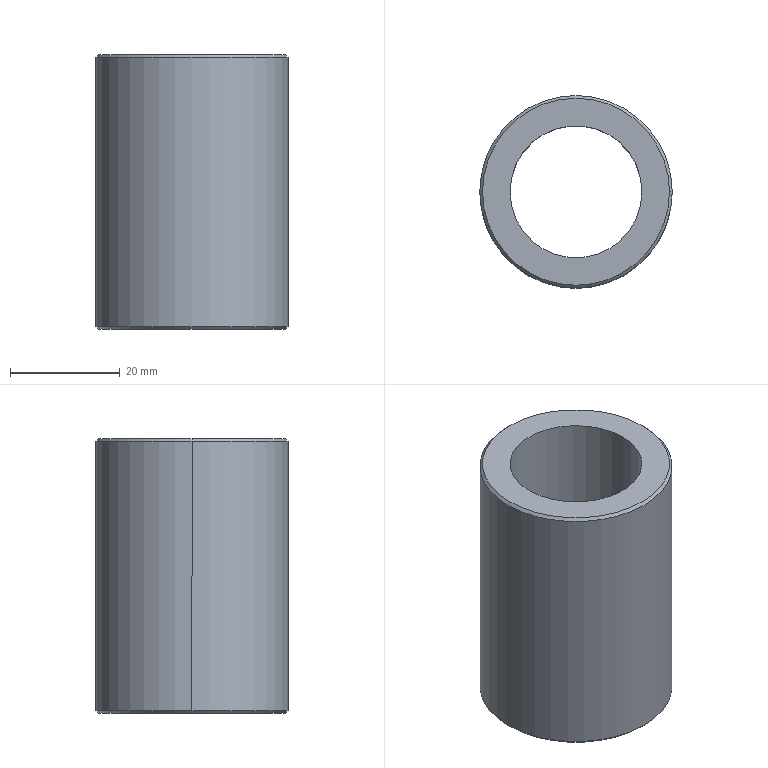Part | SolidWorks | features Revolution 1 | 1 solid | 13 faces | box 35 x 35 x 50 mm | volume 24381 mm3 | cylinder 6 | cone 4 | plane 3 | commonest cylinder face diameters 24 x2 25 x2 35 x2
STEP:
#1=CARTESIAN_POINT('',(-17.,0.,50.));
#2=VERTEX_POINT('',#1);
#3=CARTESIAN_POINT('',(17.,0.,50.));
#4=VERTEX_POINT('',#3);
#5=CARTESIAN_POINT('',(0.,0.,50.));
#6=DIRECTION('',(0.,0.,-1.));
#7=DIRECTION('',(-1.,0.,0.));
#8=AXIS2_PLACEMENT_3D('',#5,#6,#7);
#9=CIRCLE('',#8,17.);
#10=EDGE_CURVE('',#2,#4,#9,.T.);
#11=ORIENTED_EDGE('',*,*,#10,.T.);
#12=CARTESIAN_POINT('',(17.5,0.,49.5));
#13=VERTEX_POINT('',#12);
#14=CARTESIAN_POINT('',(17.5,0.,49.5));
#15=DIRECTION('',(0.7071,0.,-0.7071));
#16=VECTOR('',#15,1000.);
#17=LINE('',#14,#16);
#18=EDGE_CURVE('',#4,#13,#17,.T.);
#19=ORIENTED_EDGE('',*,*,#18,.T.);
#20=CARTESIAN_POINT('',(-17.5,0.,49.5));
#21=VERTEX_POINT('',#20);
#22=CARTESIAN_POINT('',(0.,0.,49.5));
#23=DIRECTION('',(0.,0.,-1.));
#24=DIRECTION('',(-1.,0.,0.));
#25=AXIS2_PLACEMENT_3D('',#22,#23,#24);
#26=CIRCLE('',#25,17.5);
#27=EDGE_CURVE('',#21,#13,#26,.T.);
#28=ORIENTED_EDGE('',*,*,#27,.F.);
#29=CARTESIAN_POINT('',(-17.5,0.,49.5));
#30=DIRECTION('',(-0.7071,0.,-0.7071));
#31=VECTOR('',#30,1000.);
#32=LINE('',#29,#31);
#33=EDGE_CURVE('',#2,#21,#32,.T.);
#34=ORIENTED_EDGE('',*,*,#33,.F.);
#35=EDGE_LOOP('',(#11,#19,#28,#34));
#36=FACE_OUTER_BOUND('',#35,.T.);
#37=CARTESIAN_POINT('',(0.,0.,49.5));
#38=DIRECTION('',(0.,0.,-1.));
#39=DIRECTION('',(-1.,0.,0.));
#40=AXIS2_PLACEMENT_3D('',#37,#38,#39);
#41=CONICAL_SURFACE('',#40,17.5,0.7854);
#42=ADVANCED_FACE('',(#36),#41,.T.);
#43=ORIENTED_EDGE('',*,*,#27,.T.);
#44=CARTESIAN_POINT('',(17.5,0.,0.5));
#45=VERTEX_POINT('',#44);
#46=CARTESIAN_POINT('',(17.5,0.,50.));
#47=DIRECTION('',(0.,0.,-1.));
#48=VECTOR('',#47,1000.);
#49=LINE('',#46,#48);
#50=EDGE_CURVE('',#13,#45,#49,.T.);
#51=ORIENTED_EDGE('',*,*,#50,.T.);
#52=CARTESIAN_POINT('',(-17.5,0.,0.5));
#53=VERTEX_POINT('',#52);
#54=CARTESIAN_POINT('',(0.,0.,0.5));
#55=DIRECTION('',(0.,0.,-1.));
#56=DIRECTION('',(-1.,0.,0.));
#57=AXIS2_PLACEMENT_3D('',#54,#55,#56);
#58=CIRCLE('',#57,17.5);
#59=EDGE_CURVE('',#53,#45,#58,.T.);
#60=ORIENTED_EDGE('',*,*,#59,.F.);
#61=CARTESIAN_POINT('',(-17.5,0.,50.));
#62=DIRECTION('',(0.,0.,-1.));
#63=VECTOR('',#62,1000.);
#64=LINE('',#61,#63);
#65=EDGE_CURVE('',#21,#53,#64,.T.);
#66=ORIENTED_EDGE('',*,*,#65,.F.);
#67=EDGE_LOOP('',(#43,#51,#60,#66));
#68=FACE_OUTER_BOUND('',#67,.T.);
#69=CARTESIAN_POINT('',(0.,0.,50.));
#70=DIRECTION('',(0.,0.,-1.));
#71=DIRECTION('',(-1.,0.,0.));
#72=AXIS2_PLACEMENT_3D('',#69,#70,#71);
#73=CYLINDRICAL_SURFACE('',#72,17.5);
#74=ADVANCED_FACE('',(#68),#73,.T.);
#75=CARTESIAN_POINT('',(-17.,0.,0.));
#76=VERTEX_POINT('',#75);
#77=CARTESIAN_POINT('',(17.,0.,0.));
#78=VERTEX_POINT('',#77);
#79=CARTESIAN_POINT('',(0.,0.,0.));
#80=DIRECTION('',(0.,0.,-1.));
#81=DIRECTION('',(-1.,0.,0.));
#82=AXIS2_PLACEMENT_3D('',#79,#80,#81);
#83=CIRCLE('',#82,17.);
#84=EDGE_CURVE('',#76,#78,#83,.T.);
#85=ORIENTED_EDGE('',*,*,#84,.F.);
#86=CARTESIAN_POINT('',(-17.,0.,0.));
#87=DIRECTION('',(-0.7071,0.,0.7071));
#88=VECTOR('',#87,1000.);
#89=LINE('',#86,#88);
#90=EDGE_CURVE('',#76,#53,#89,.T.);
#91=ORIENTED_EDGE('',*,*,#90,.T.);
#92=ORIENTED_EDGE('',*,*,#59,.T.);
#93=CARTESIAN_POINT('',(17.,0.,0.));
#94=DIRECTION('',(0.7071,0.,0.7071));
#95=VECTOR('',#94,1000.);
#96=LINE('',#93,#95);
#97=EDGE_CURVE('',#78,#45,#96,.T.);
#98=ORIENTED_EDGE('',*,*,#97,.F.);
#99=EDGE_LOOP('',(#85,#91,#92,#98));
#100=FACE_OUTER_BOUND('',#99,.T.);
#101=CARTESIAN_POINT('',(0.,0.,0.));
#102=DIRECTION('',(0.,0.,1.));
#103=DIRECTION('',(1.,0.,0.));
#104=AXIS2_PLACEMENT_3D('',#101,#102,#103);
#105=CONICAL_SURFACE('',#104,17.,0.7854);
#106=ADVANCED_FACE('',(#100),#105,.T.);
#107=CARTESIAN_POINT('',(12.5,0.,28.));
#108=VERTEX_POINT('',#107);
#109=CARTESIAN_POINT('',(-12.5,0.,28.));
#110=VERTEX_POINT('',#109);
#111=CARTESIAN_POINT('',(0.,0.,28.));
#112=DIRECTION('',(0.,0.,-1.));
#113=DIRECTION('',(-1.,0.,0.));
#114=AXIS2_PLACEMENT_3D('',#111,#112,#113);
#115=CIRCLE('',#114,12.5);
#116=EDGE_CURVE('',#108,#110,#115,.T.);
#117=ORIENTED_EDGE('',*,*,#116,.F.);
#118=CARTESIAN_POINT('',(12.5,0.,0.));
#119=VERTEX_POINT('',#118);
#120=CARTESIAN_POINT('',(12.5,0.,50.));
#121=DIRECTION('',(0.,0.,-1.));
#122=VECTOR('',#121,1000.);
#123=LINE('',#120,#122);
#124=EDGE_CURVE('',#108,#119,#123,.T.);
#125=ORIENTED_EDGE('',*,*,#124,.T.);
#126=CARTESIAN_POINT('',(-12.5,0.,0.));
#127=VERTEX_POINT('',#126);
#128=CARTESIAN_POINT('',(0.,0.,0.));
#129=DIRECTION('',(0.,0.,-1.));
#130=DIRECTION('',(-1.,0.,0.));
#131=AXIS2_PLACEMENT_3D('',#128,#129,#130);
#132=CIRCLE('',#131,12.5);
#133=EDGE_CURVE('',#119,#127,#132,.T.);
#134=ORIENTED_EDGE('',*,*,#133,.T.);
#135=CARTESIAN_POINT('',(-12.5,0.,50.));
#136=DIRECTION('',(0.,0.,-1.));
#137=VECTOR('',#136,1000.);
#138=LINE('',#135,#137);
#139=EDGE_CURVE('',#110,#127,#138,.T.);
#140=ORIENTED_EDGE('',*,*,#139,.F.);
#141=EDGE_LOOP('',(#117,#125,#134,#140));
#142=FACE_OUTER_BOUND('',#141,.T.);
#143=CARTESIAN_POINT('',(0.,0.,50.));
#144=DIRECTION('',(0.,0.,-1.));
#145=DIRECTION('',(-1.,0.,0.));
#146=AXIS2_PLACEMENT_3D('',#143,#144,#145);
#147=CYLINDRICAL_SURFACE('',#146,12.5);
#148=ADVANCED_FACE('',(#142),#147,.F.);
#149=CARTESIAN_POINT('',(12.,0.,50.));
#150=VERTEX_POINT('',#149);
#151=CARTESIAN_POINT('',(-12.,0.,50.));
#152=VERTEX_POINT('',#151);
#153=CARTESIAN_POINT('',(0.,0.,50.));
#154=DIRECTION('',(0.,0.,-1.));
#155=DIRECTION('',(-1.,0.,0.));
#156=AXIS2_PLACEMENT_3D('',#153,#154,#155);
#157=CIRCLE('',#156,12.);
#158=EDGE_CURVE('',#150,#152,#157,.T.);
#159=ORIENTED_EDGE('',*,*,#158,.F.);
#160=CARTESIAN_POINT('',(12.,0.,28.));
#161=VERTEX_POINT('',#160);
#162=CARTESIAN_POINT('',(12.,0.,50.));
#163=DIRECTION('',(0.,0.,-1.));
#164=VECTOR('',#163,1000.);
#165=LINE('',#162,#164);
#166=EDGE_CURVE('',#150,#161,#165,.T.);
#167=ORIENTED_EDGE('',*,*,#166,.T.);
#168=CARTESIAN_POINT('',(-12.,0.,28.));
#169=VERTEX_POINT('',#168);
#170=CARTESIAN_POINT('',(0.,0.,28.));
#171=DIRECTION('',(0.,0.,-1.));
#172=DIRECTION('',(-1.,0.,0.));
#173=AXIS2_PLACEMENT_3D('',#170,#171,#172);
#174=CIRCLE('',#173,12.);
#175=EDGE_CURVE('',#161,#169,#174,.T.);
#176=ORIENTED_EDGE('',*,*,#175,.T.);
#177=CARTESIAN_POINT('',(-12.,0.,50.));
#178=DIRECTION('',(0.,0.,-1.));
#179=VECTOR('',#178,1000.);
#180=LINE('',#177,#179);
#181=EDGE_CURVE('',#152,#169,#180,.T.);
#182=ORIENTED_EDGE('',*,*,#181,.F.);
#183=EDGE_LOOP('',(#159,#167,#176,#182));
#184=FACE_OUTER_BOUND('',#183,.T.);
#185=CARTESIAN_POINT('',(0.,0.,50.));
#186=DIRECTION('',(0.,0.,-1.));
#187=DIRECTION('',(-1.,0.,0.));
#188=AXIS2_PLACEMENT_3D('',#185,#186,#187);
#189=CYLINDRICAL_SURFACE('',#188,12.);
#190=ADVANCED_FACE('',(#184),#189,.F.);
#191=ORIENTED_EDGE('',*,*,#166,.F.);
#192=CARTESIAN_POINT('',(0.,0.,50.));
#193=DIRECTION('',(0.,0.,-1.));
#194=DIRECTION('',(-1.,0.,0.));
#195=AXIS2_PLACEMENT_3D('',#192,#193,#194);
#196=CIRCLE('',#195,12.);
#197=EDGE_CURVE('',#152,#150,#196,.T.);
#198=ORIENTED_EDGE('',*,*,#197,.F.);
#199=ORIENTED_EDGE('',*,*,#181,.T.);
#200=CARTESIAN_POINT('',(0.,0.,28.));
#201=DIRECTION('',(0.,0.,-1.));
#202=DIRECTION('',(-1.,0.,0.));
#203=AXIS2_PLACEMENT_3D('',#200,#201,#202);
#204=CIRCLE('',#203,12.);
#205=EDGE_CURVE('',#169,#161,#204,.T.);
#206=ORIENTED_EDGE('',*,*,#205,.T.);
#207=EDGE_LOOP('',(#191,#198,#199,#206));
#208=FACE_OUTER_BOUND('',#207,.T.);
#209=CARTESIAN_POINT('',(0.,0.,50.));
#210=DIRECTION('',(0.,0.,-1.));
#211=DIRECTION('',(-1.,0.,0.));
#212=AXIS2_PLACEMENT_3D('',#209,#210,#211);
#213=CYLINDRICAL_SURFACE('',#212,12.);
#214=ADVANCED_FACE('',(#208),#213,.F.);
#215=CARTESIAN_POINT('',(0.,0.,28.));
#216=DIRECTION('',(0.,0.,-1.));
#217=DIRECTION('',(-1.,0.,0.));
#218=AXIS2_PLACEMENT_3D('',#215,#216,#217);
#219=CIRCLE('',#218,12.5);
#220=EDGE_CURVE('',#110,#108,#219,.T.);
#221=ORIENTED_EDGE('',*,*,#220,.T.);
#222=ORIENTED_EDGE('',*,*,#116,.T.);
#223=EDGE_LOOP('',(#221,#222));
#224=FACE_OUTER_BOUND('',#223,.T.);
#225=ORIENTED_EDGE('',*,*,#205,.F.);
#226=ORIENTED_EDGE('',*,*,#175,.F.);
#227=EDGE_LOOP('',(#225,#226));
#228=FACE_BOUND('',#227,.T.);
#229=CARTESIAN_POINT('',(12.,0.,28.));
#230=DIRECTION('',(0.,0.,-1.));
#231=DIRECTION('',(-1.,0.,0.));
#232=AXIS2_PLACEMENT_3D('',#229,#230,#231);
#233=PLANE('',#232);
#234=ADVANCED_FACE('',(#224,#228),#233,.T.);
#235=ORIENTED_EDGE('',*,*,#124,.F.);
#236=ORIENTED_EDGE('',*,*,#220,.F.);
#237=ORIENTED_EDGE('',*,*,#139,.T.);
#238=CARTESIAN_POINT('',(0.,0.,0.));
#239=DIRECTION('',(0.,0.,-1.));
#240=DIRECTION('',(-1.,0.,0.));
#241=AXIS2_PLACEMENT_3D('',#238,#239,#240);
#242=CIRCLE('',#241,12.5);
#243=EDGE_CURVE('',#127,#119,#242,.T.);
#244=ORIENTED_EDGE('',*,*,#243,.T.);
#245=EDGE_LOOP('',(#235,#236,#237,#244));
#246=FACE_OUTER_BOUND('',#245,.T.);
#247=CARTESIAN_POINT('',(0.,0.,50.));
#248=DIRECTION('',(0.,0.,-1.));
#249=DIRECTION('',(-1.,0.,0.));
#250=AXIS2_PLACEMENT_3D('',#247,#248,#249);
#251=CYLINDRICAL_SURFACE('',#250,12.5);
#252=ADVANCED_FACE('',(#246),#251,.F.);
#253=CARTESIAN_POINT('',(0.,0.,0.));
#254=DIRECTION('',(0.,0.,-1.));
#255=DIRECTION('',(-1.,0.,0.));
#256=AXIS2_PLACEMENT_3D('',#253,#254,#255);
#257=CIRCLE('',#256,17.);
#258=EDGE_CURVE('',#78,#76,#257,.T.);
#259=ORIENTED_EDGE('',*,*,#258,.T.);
#260=ORIENTED_EDGE('',*,*,#84,.T.);
#261=EDGE_LOOP('',(#259,#260));
#262=FACE_OUTER_BOUND('',#261,.T.);
#263=ORIENTED_EDGE('',*,*,#243,.F.);
#264=ORIENTED_EDGE('',*,*,#133,.F.);
#265=EDGE_LOOP('',(#263,#264));
#266=FACE_BOUND('',#265,.T.);
#267=CARTESIAN_POINT('',(12.5,0.,0.));
#268=DIRECTION('',(0.,0.,-1.));
#269=DIRECTION('',(-1.,0.,0.));
#270=AXIS2_PLACEMENT_3D('',#267,#268,#269);
#271=PLANE('',#270);
#272=ADVANCED_FACE('',(#262,#266),#271,.T.);
#273=ORIENTED_EDGE('',*,*,#90,.F.);
#274=ORIENTED_EDGE('',*,*,#258,.F.);
#275=ORIENTED_EDGE('',*,*,#97,.T.);
#276=CARTESIAN_POINT('',(0.,0.,0.5));
#277=DIRECTION('',(0.,0.,-1.));
#278=DIRECTION('',(-1.,0.,0.));
#279=AXIS2_PLACEMENT_3D('',#276,#277,#278);
#280=CIRCLE('',#279,17.5);
#281=EDGE_CURVE('',#45,#53,#280,.T.);
#282=ORIENTED_EDGE('',*,*,#281,.T.);
#283=EDGE_LOOP('',(#273,#274,#275,#282));
#284=FACE_OUTER_BOUND('',#283,.T.);
#285=CARTESIAN_POINT('',(0.,0.,0.));
#286=DIRECTION('',(0.,0.,1.));
#287=DIRECTION('',(1.,0.,0.));
#288=AXIS2_PLACEMENT_3D('',#285,#286,#287);
#289=CONICAL_SURFACE('',#288,17.,0.7854);
#290=ADVANCED_FACE('',(#284),#289,.T.);
#291=ORIENTED_EDGE('',*,*,#50,.F.);
#292=CARTESIAN_POINT('',(0.,0.,49.5));
#293=DIRECTION('',(0.,0.,-1.));
#294=DIRECTION('',(-1.,0.,0.));
#295=AXIS2_PLACEMENT_3D('',#292,#293,#294);
#296=CIRCLE('',#295,17.5);
#297=EDGE_CURVE('',#13,#21,#296,.T.);
#298=ORIENTED_EDGE('',*,*,#297,.T.);
#299=ORIENTED_EDGE('',*,*,#65,.T.);
#300=ORIENTED_EDGE('',*,*,#281,.F.);
#301=EDGE_LOOP('',(#291,#298,#299,#300));
#302=FACE_OUTER_BOUND('',#301,.T.);
#303=CARTESIAN_POINT('',(0.,0.,50.));
#304=DIRECTION('',(0.,0.,-1.));
#305=DIRECTION('',(-1.,0.,0.));
#306=AXIS2_PLACEMENT_3D('',#303,#304,#305);
#307=CYLINDRICAL_SURFACE('',#306,17.5);
#308=ADVANCED_FACE('',(#302),#307,.T.);
#309=ORIENTED_EDGE('',*,*,#18,.F.);
#310=CARTESIAN_POINT('',(0.,0.,50.));
#311=DIRECTION('',(0.,0.,-1.));
#312=DIRECTION('',(-1.,0.,0.));
#313=AXIS2_PLACEMENT_3D('',#310,#311,#312);
#314=CIRCLE('',#313,17.);
#315=EDGE_CURVE('',#4,#2,#314,.T.);
#316=ORIENTED_EDGE('',*,*,#315,.T.);
#317=ORIENTED_EDGE('',*,*,#33,.T.);
#318=ORIENTED_EDGE('',*,*,#297,.F.);
#319=EDGE_LOOP('',(#309,#316,#317,#318));
#320=FACE_OUTER_BOUND('',#319,.T.);
#321=CARTESIAN_POINT('',(0.,0.,49.5));
#322=DIRECTION('',(0.,0.,-1.));
#323=DIRECTION('',(-1.,0.,0.));
#324=AXIS2_PLACEMENT_3D('',#321,#322,#323);
#325=CONICAL_SURFACE('',#324,17.5,0.7854);
#326=ADVANCED_FACE('',(#320),#325,.T.);
#327=ORIENTED_EDGE('',*,*,#197,.T.);
#328=ORIENTED_EDGE('',*,*,#158,.T.);
#329=EDGE_LOOP('',(#327,#328));
#330=FACE_BOUND('',#329,.T.);
#331=ORIENTED_EDGE('',*,*,#10,.F.);
#332=ORIENTED_EDGE('',*,*,#315,.F.);
#333=EDGE_LOOP('',(#331,#332));
#334=FACE_OUTER_BOUND('',#333,.T.);
#335=CARTESIAN_POINT('',(17.,0.,50.));
#336=DIRECTION('',(0.,0.,1.));
#337=DIRECTION('',(1.,0.,0.));
#338=AXIS2_PLACEMENT_3D('',#335,#336,#337);
#339=PLANE('',#338);
#340=ADVANCED_FACE('',(#330,#334),#339,.T.);
#341=CLOSED_SHELL('',(#42,#74,#106,#148,#190,#214,#234,#252,#272,#290,#308,#326,#340));
#342=MANIFOLD_SOLID_BREP('',#341);
#343=CARTESIAN_POINT('',(0.,0.,0.));
#344=DIRECTION('',(0.,0.,1.));
#345=DIRECTION('',(1.,0.,0.));
#346=AXIS2_PLACEMENT_3D('',#343,#344,#345);
#347=(LENGTH_UNIT()NAMED_UNIT(*)SI_UNIT(.MILLI.,.METRE.));
#348=UNCERTAINTY_MEASURE_WITH_UNIT(LENGTH_MEASURE(0.00001),#347,'','');
#349=(NAMED_UNIT(*)PLANE_ANGLE_UNIT()SI_UNIT($,.RADIAN.));
#350=(NAMED_UNIT(*)SI_UNIT($,.STERADIAN.)SOLID_ANGLE_UNIT());
#351=(GEOMETRIC_REPRESENTATION_CONTEXT(3)GLOBAL_UNCERTAINTY_ASSIGNED_CONTEXT((#348))GLOBAL_UNIT_ASSIGNED_CONTEXT((#347,#349,#350))REPRESENTATION_CONTEXT('',''));
#352=ADVANCED_BREP_SHAPE_REPRESENTATION('',(#342,#346),#351);